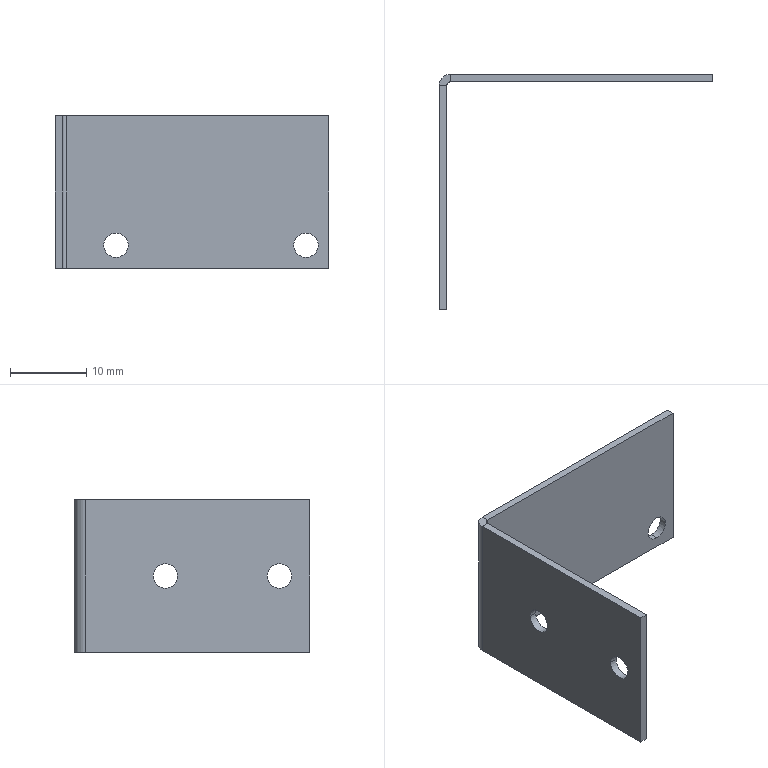Part | SolidWorks | features ICE 2, FlatPattern 1, SMBaseFlange 1, SheetMetal 1 | 1 solid | 22 faces | box 36 x 31 x 20 mm | volume 1279 mm3 | plane 12 | cylinder 10 | commonest cylinder face diameters 3.2 x8 1 x1 3 x1
STEP:
#1=CARTESIAN_POINT('',(-1.,-12.6,10.));
#2=VERTEX_POINT('',#1);
#3=CARTESIAN_POINT('',(-1.,-9.4,10.));
#4=VERTEX_POINT('',#3);
#5=CARTESIAN_POINT('',(-1.,-11.,10.));
#6=DIRECTION('',(1.,0.,0.));
#7=DIRECTION('',(0.,1.,0.));
#8=AXIS2_PLACEMENT_3D('',#5,#6,#7);
#9=CIRCLE('',#8,1.6);
#10=EDGE_CURVE('',#2,#4,#9,.T.);
#11=ORIENTED_EDGE('',*,*,#10,.F.);
#12=CARTESIAN_POINT('',(0.,-12.6,10.));
#13=VERTEX_POINT('',#12);
#14=CARTESIAN_POINT('',(-1.,-12.6,10.));
#15=DIRECTION('',(1.,0.,0.));
#16=VECTOR('',#15,1000.);
#17=LINE('',#14,#16);
#18=EDGE_CURVE('',#2,#13,#17,.T.);
#19=ORIENTED_EDGE('',*,*,#18,.T.);
#20=CARTESIAN_POINT('',(0.,-9.4,10.));
#21=VERTEX_POINT('',#20);
#22=CARTESIAN_POINT('',(0.,-11.,10.));
#23=DIRECTION('',(1.,0.,0.));
#24=DIRECTION('',(0.,1.,0.));
#25=AXIS2_PLACEMENT_3D('',#22,#23,#24);
#26=CIRCLE('',#25,1.6);
#27=EDGE_CURVE('',#13,#21,#26,.T.);
#28=ORIENTED_EDGE('',*,*,#27,.T.);
#29=CARTESIAN_POINT('',(-1.,-9.4,10.));
#30=DIRECTION('',(1.,0.,0.));
#31=VECTOR('',#30,1000.);
#32=LINE('',#29,#31);
#33=EDGE_CURVE('',#4,#21,#32,.T.);
#34=ORIENTED_EDGE('',*,*,#33,.F.);
#35=EDGE_LOOP('',(#11,#19,#28,#34));
#36=FACE_OUTER_BOUND('',#35,.T.);
#37=CARTESIAN_POINT('',(-1.,-11.,10.));
#38=DIRECTION('',(1.,0.,0.));
#39=DIRECTION('',(0.,1.,0.));
#40=AXIS2_PLACEMENT_3D('',#37,#38,#39);
#41=CYLINDRICAL_SURFACE('',#40,1.6);
#42=ADVANCED_FACE('',(#36),#41,.F.);
#43=CARTESIAN_POINT('',(-1.,-27.6,10.));
#44=VERTEX_POINT('',#43);
#45=CARTESIAN_POINT('',(-1.,-24.4,10.));
#46=VERTEX_POINT('',#45);
#47=CARTESIAN_POINT('',(-1.,-26.,10.));
#48=DIRECTION('',(1.,0.,0.));
#49=DIRECTION('',(0.,1.,0.));
#50=AXIS2_PLACEMENT_3D('',#47,#48,#49);
#51=CIRCLE('',#50,1.6);
#52=EDGE_CURVE('',#44,#46,#51,.T.);
#53=ORIENTED_EDGE('',*,*,#52,.F.);
#54=CARTESIAN_POINT('',(0.,-27.6,10.));
#55=VERTEX_POINT('',#54);
#56=CARTESIAN_POINT('',(-1.,-27.6,10.));
#57=DIRECTION('',(1.,0.,0.));
#58=VECTOR('',#57,1000.);
#59=LINE('',#56,#58);
#60=EDGE_CURVE('',#44,#55,#59,.T.);
#61=ORIENTED_EDGE('',*,*,#60,.T.);
#62=CARTESIAN_POINT('',(0.,-24.4,10.));
#63=VERTEX_POINT('',#62);
#64=CARTESIAN_POINT('',(0.,-26.,10.));
#65=DIRECTION('',(1.,0.,0.));
#66=DIRECTION('',(0.,1.,0.));
#67=AXIS2_PLACEMENT_3D('',#64,#65,#66);
#68=CIRCLE('',#67,1.6);
#69=EDGE_CURVE('',#55,#63,#68,.T.);
#70=ORIENTED_EDGE('',*,*,#69,.T.);
#71=CARTESIAN_POINT('',(-1.,-24.4,10.));
#72=DIRECTION('',(1.,0.,0.));
#73=VECTOR('',#72,1000.);
#74=LINE('',#71,#73);
#75=EDGE_CURVE('',#46,#63,#74,.T.);
#76=ORIENTED_EDGE('',*,*,#75,.F.);
#77=EDGE_LOOP('',(#53,#61,#70,#76));
#78=FACE_OUTER_BOUND('',#77,.T.);
#79=CARTESIAN_POINT('',(-1.,-26.,10.));
#80=DIRECTION('',(1.,0.,0.));
#81=DIRECTION('',(0.,1.,0.));
#82=AXIS2_PLACEMENT_3D('',#79,#80,#81);
#83=CYLINDRICAL_SURFACE('',#82,1.6);
#84=ADVANCED_FACE('',(#78),#83,.F.);
#85=CARTESIAN_POINT('',(7.,0.,4.6));
#86=VERTEX_POINT('',#85);
#87=CARTESIAN_POINT('',(7.,0.,1.4));
#88=VERTEX_POINT('',#87);
#89=CARTESIAN_POINT('',(7.,0.,3.));
#90=DIRECTION('',(0.,-1.,0.));
#91=DIRECTION('',(0.,0.,-1.));
#92=AXIS2_PLACEMENT_3D('',#89,#90,#91);
#93=CIRCLE('',#92,1.6);
#94=EDGE_CURVE('',#86,#88,#93,.T.);
#95=ORIENTED_EDGE('',*,*,#94,.T.);
#96=CARTESIAN_POINT('',(7.,1.,1.4));
#97=VERTEX_POINT('',#96);
#98=CARTESIAN_POINT('',(7.,-9.,1.4));
#99=DIRECTION('',(0.,1.,0.));
#100=VECTOR('',#99,1000.);
#101=LINE('',#98,#100);
#102=EDGE_CURVE('',#88,#97,#101,.T.);
#103=ORIENTED_EDGE('',*,*,#102,.T.);
#104=CARTESIAN_POINT('',(7.,1.,4.6));
#105=VERTEX_POINT('',#104);
#106=CARTESIAN_POINT('',(7.,1.,3.));
#107=DIRECTION('',(0.,1.,0.));
#108=DIRECTION('',(0.,0.,1.));
#109=AXIS2_PLACEMENT_3D('',#106,#107,#108);
#110=CIRCLE('',#109,1.6);
#111=EDGE_CURVE('',#97,#105,#110,.T.);
#112=ORIENTED_EDGE('',*,*,#111,.T.);
#113=CARTESIAN_POINT('',(7.,-9.,4.6));
#114=DIRECTION('',(0.,1.,0.));
#115=VECTOR('',#114,1000.);
#116=LINE('',#113,#115);
#117=EDGE_CURVE('',#86,#105,#116,.T.);
#118=ORIENTED_EDGE('',*,*,#117,.F.);
#119=EDGE_LOOP('',(#95,#103,#112,#118));
#120=FACE_OUTER_BOUND('',#119,.T.);
#121=CARTESIAN_POINT('',(7.,-9.,3.));
#122=DIRECTION('',(0.,1.,0.));
#123=DIRECTION('',(0.,0.,1.));
#124=AXIS2_PLACEMENT_3D('',#121,#122,#123);
#125=CYLINDRICAL_SURFACE('',#124,1.6);
#126=ADVANCED_FACE('',(#120),#125,.F.);
#127=CARTESIAN_POINT('',(32.,0.,4.6));
#128=VERTEX_POINT('',#127);
#129=CARTESIAN_POINT('',(32.,0.,1.4));
#130=VERTEX_POINT('',#129);
#131=CARTESIAN_POINT('',(32.,0.,3.));
#132=DIRECTION('',(0.,-1.,0.));
#133=DIRECTION('',(0.,0.,-1.));
#134=AXIS2_PLACEMENT_3D('',#131,#132,#133);
#135=CIRCLE('',#134,1.6);
#136=EDGE_CURVE('',#128,#130,#135,.T.);
#137=ORIENTED_EDGE('',*,*,#136,.T.);
#138=CARTESIAN_POINT('',(32.,1.,1.4));
#139=VERTEX_POINT('',#138);
#140=CARTESIAN_POINT('',(32.,-9.,1.4));
#141=DIRECTION('',(0.,1.,0.));
#142=VECTOR('',#141,1000.);
#143=LINE('',#140,#142);
#144=EDGE_CURVE('',#130,#139,#143,.T.);
#145=ORIENTED_EDGE('',*,*,#144,.T.);
#146=CARTESIAN_POINT('',(32.,1.,4.6));
#147=VERTEX_POINT('',#146);
#148=CARTESIAN_POINT('',(32.,1.,3.));
#149=DIRECTION('',(0.,1.,0.));
#150=DIRECTION('',(0.,0.,1.));
#151=AXIS2_PLACEMENT_3D('',#148,#149,#150);
#152=CIRCLE('',#151,1.6);
#153=EDGE_CURVE('',#139,#147,#152,.T.);
#154=ORIENTED_EDGE('',*,*,#153,.T.);
#155=CARTESIAN_POINT('',(32.,-9.,4.6));
#156=DIRECTION('',(0.,1.,0.));
#157=VECTOR('',#156,1000.);
#158=LINE('',#155,#157);
#159=EDGE_CURVE('',#128,#147,#158,.T.);
#160=ORIENTED_EDGE('',*,*,#159,.F.);
#161=EDGE_LOOP('',(#137,#145,#154,#160));
#162=FACE_OUTER_BOUND('',#161,.T.);
#163=CARTESIAN_POINT('',(32.,-9.,3.));
#164=DIRECTION('',(0.,1.,0.));
#165=DIRECTION('',(0.,0.,1.));
#166=AXIS2_PLACEMENT_3D('',#163,#164,#165);
#167=CYLINDRICAL_SURFACE('',#166,1.6);
#168=ADVANCED_FACE('',(#162),#167,.F.);
#169=CARTESIAN_POINT('',(0.,-0.5,20.));
#170=VERTEX_POINT('',#169);
#171=CARTESIAN_POINT('',(-1.,-0.5,20.));
#172=VERTEX_POINT('',#171);
#173=CARTESIAN_POINT('',(0.,-0.5,20.));
#174=DIRECTION('',(-1.,0.,0.));
#175=VECTOR('',#174,1000.);
#176=LINE('',#173,#175);
#177=EDGE_CURVE('',#170,#172,#176,.T.);
#178=ORIENTED_EDGE('',*,*,#177,.F.);
#179=CARTESIAN_POINT('',(0.5,0.,20.));
#180=VERTEX_POINT('',#179);
#181=CARTESIAN_POINT('',(0.5,-0.5,20.));
#182=DIRECTION('',(0.,0.,1.));
#183=DIRECTION('',(-1.,0.,0.));
#184=AXIS2_PLACEMENT_3D('',#181,#182,#183);
#185=CIRCLE('',#184,0.5);
#186=EDGE_CURVE('',#180,#170,#185,.T.);
#187=ORIENTED_EDGE('',*,*,#186,.F.);
#188=CARTESIAN_POINT('',(0.5,1.,20.));
#189=VERTEX_POINT('',#188);
#190=CARTESIAN_POINT('',(0.5,1.,20.));
#191=DIRECTION('',(0.,-1.,0.));
#192=VECTOR('',#191,1000.);
#193=LINE('',#190,#192);
#194=EDGE_CURVE('',#189,#180,#193,.T.);
#195=ORIENTED_EDGE('',*,*,#194,.F.);
#196=CARTESIAN_POINT('',(0.5,-0.5,20.));
#197=DIRECTION('',(0.,0.,1.));
#198=DIRECTION('',(1.,0.,0.));
#199=AXIS2_PLACEMENT_3D('',#196,#197,#198);
#200=CIRCLE('',#199,1.5);
#201=EDGE_CURVE('',#189,#172,#200,.T.);
#202=ORIENTED_EDGE('',*,*,#201,.T.);
#203=EDGE_LOOP('',(#178,#187,#195,#202));
#204=FACE_OUTER_BOUND('',#203,.T.);
#205=CARTESIAN_POINT('',(0.,-0.5,20.));
#206=DIRECTION('',(0.,0.,1.));
#207=DIRECTION('',(1.,0.,0.));
#208=AXIS2_PLACEMENT_3D('',#205,#206,#207);
#209=PLANE('',#208);
#210=ADVANCED_FACE('',(#204),#209,.T.);
#211=CARTESIAN_POINT('',(0.,-30.,20.));
#212=VERTEX_POINT('',#211);
#213=CARTESIAN_POINT('',(0.,0.,20.));
#214=DIRECTION('',(0.,-1.,0.));
#215=VECTOR('',#214,1000.);
#216=LINE('',#213,#215);
#217=EDGE_CURVE('',#170,#212,#216,.T.);
#218=ORIENTED_EDGE('',*,*,#217,.F.);
#219=ORIENTED_EDGE('',*,*,#177,.T.);
#220=CARTESIAN_POINT('',(-1.,-30.,20.));
#221=VERTEX_POINT('',#220);
#222=CARTESIAN_POINT('',(-1.,0.,20.));
#223=DIRECTION('',(0.,-1.,0.));
#224=VECTOR('',#223,1000.);
#225=LINE('',#222,#224);
#226=EDGE_CURVE('',#172,#221,#225,.T.);
#227=ORIENTED_EDGE('',*,*,#226,.T.);
#228=CARTESIAN_POINT('',(0.,-30.,20.));
#229=DIRECTION('',(-1.,0.,0.));
#230=VECTOR('',#229,1000.);
#231=LINE('',#228,#230);
#232=EDGE_CURVE('',#212,#221,#231,.T.);
#233=ORIENTED_EDGE('',*,*,#232,.F.);
#234=EDGE_LOOP('',(#218,#219,#227,#233));
#235=FACE_OUTER_BOUND('',#234,.T.);
#236=CARTESIAN_POINT('',(0.5,1.,20.));
#237=DIRECTION('',(0.,0.,1.));
#238=DIRECTION('',(1.,0.,0.));
#239=AXIS2_PLACEMENT_3D('',#236,#237,#238);
#240=PLANE('',#239);
#241=ADVANCED_FACE('',(#235),#240,.T.);
#242=CARTESIAN_POINT('',(0.5,0.,0.));
#243=VERTEX_POINT('',#242);
#244=CARTESIAN_POINT('',(0.5,1.,0.));
#245=VERTEX_POINT('',#244);
#246=CARTESIAN_POINT('',(0.5,0.,0.));
#247=DIRECTION('',(0.,1.,0.));
#248=VECTOR('',#247,1000.);
#249=LINE('',#246,#248);
#250=EDGE_CURVE('',#243,#245,#249,.T.);
#251=ORIENTED_EDGE('',*,*,#250,.F.);
#252=CARTESIAN_POINT('',(0.,-0.5,0.));
#253=VERTEX_POINT('',#252);
#254=CARTESIAN_POINT('',(0.5,-0.5,0.));
#255=DIRECTION('',(0.,0.,1.));
#256=DIRECTION('',(-1.,0.,0.));
#257=AXIS2_PLACEMENT_3D('',#254,#255,#256);
#258=CIRCLE('',#257,0.5);
#259=EDGE_CURVE('',#243,#253,#258,.T.);
#260=ORIENTED_EDGE('',*,*,#259,.T.);
#261=CARTESIAN_POINT('',(-1.,-0.5,0.));
#262=VERTEX_POINT('',#261);
#263=CARTESIAN_POINT('',(-1.,-0.5,0.));
#264=DIRECTION('',(1.,0.,0.));
#265=VECTOR('',#264,1000.);
#266=LINE('',#263,#265);
#267=EDGE_CURVE('',#262,#253,#266,.T.);
#268=ORIENTED_EDGE('',*,*,#267,.F.);
#269=CARTESIAN_POINT('',(0.5,-0.5,0.));
#270=DIRECTION('',(0.,0.,1.));
#271=DIRECTION('',(1.,0.,0.));
#272=AXIS2_PLACEMENT_3D('',#269,#270,#271);
#273=CIRCLE('',#272,1.5);
#274=EDGE_CURVE('',#245,#262,#273,.T.);
#275=ORIENTED_EDGE('',*,*,#274,.F.);
#276=EDGE_LOOP('',(#251,#260,#268,#275));
#277=FACE_OUTER_BOUND('',#276,.T.);
#278=CARTESIAN_POINT('',(0.5,0.,0.));
#279=DIRECTION('',(0.,0.,-1.));
#280=DIRECTION('',(-1.,0.,0.));
#281=AXIS2_PLACEMENT_3D('',#278,#279,#280);
#282=PLANE('',#281);
#283=ADVANCED_FACE('',(#277),#282,.T.);
#284=CARTESIAN_POINT('',(35.,0.,0.));
#285=VERTEX_POINT('',#284);
#286=CARTESIAN_POINT('',(0.,0.,0.));
#287=DIRECTION('',(-1.,0.,0.));
#288=VECTOR('',#287,1000.);
#289=LINE('',#286,#288);
#290=EDGE_CURVE('',#285,#243,#289,.T.);
#291=ORIENTED_EDGE('',*,*,#290,.T.);
#292=ORIENTED_EDGE('',*,*,#250,.T.);
#293=CARTESIAN_POINT('',(35.,1.,0.));
#294=VERTEX_POINT('',#293);
#295=CARTESIAN_POINT('',(0.,1.,0.));
#296=DIRECTION('',(-1.,0.,0.));
#297=VECTOR('',#296,1000.);
#298=LINE('',#295,#297);
#299=EDGE_CURVE('',#294,#245,#298,.T.);
#300=ORIENTED_EDGE('',*,*,#299,.F.);
#301=CARTESIAN_POINT('',(35.,1.,0.));
#302=DIRECTION('',(0.,-1.,0.));
#303=VECTOR('',#302,1000.);
#304=LINE('',#301,#303);
#305=EDGE_CURVE('',#294,#285,#304,.T.);
#306=ORIENTED_EDGE('',*,*,#305,.T.);
#307=EDGE_LOOP('',(#291,#292,#300,#306));
#308=FACE_OUTER_BOUND('',#307,.T.);
#309=CARTESIAN_POINT('',(-1.,-0.5,0.));
#310=DIRECTION('',(0.,0.,-1.));
#311=DIRECTION('',(-1.,0.,0.));
#312=AXIS2_PLACEMENT_3D('',#309,#310,#311);
#313=PLANE('',#312);
#314=ADVANCED_FACE('',(#308),#313,.T.);
#315=CARTESIAN_POINT('',(-1.,-11.,10.));
#316=DIRECTION('',(1.,0.,0.));
#317=DIRECTION('',(0.,1.,0.));
#318=AXIS2_PLACEMENT_3D('',#315,#316,#317);
#319=CIRCLE('',#318,1.6);
#320=EDGE_CURVE('',#4,#2,#319,.T.);
#321=ORIENTED_EDGE('',*,*,#320,.T.);
#322=ORIENTED_EDGE('',*,*,#10,.T.);
#323=EDGE_LOOP('',(#321,#322));
#324=FACE_BOUND('',#323,.T.);
#325=CARTESIAN_POINT('',(-1.,-26.,10.));
#326=DIRECTION('',(1.,0.,0.));
#327=DIRECTION('',(0.,1.,0.));
#328=AXIS2_PLACEMENT_3D('',#325,#326,#327);
#329=CIRCLE('',#328,1.6);
#330=EDGE_CURVE('',#46,#44,#329,.T.);
#331=ORIENTED_EDGE('',*,*,#330,.T.);
#332=ORIENTED_EDGE('',*,*,#52,.T.);
#333=EDGE_LOOP('',(#331,#332));
#334=FACE_BOUND('',#333,.T.);
#335=CARTESIAN_POINT('',(-1.,-30.,0.));
#336=VERTEX_POINT('',#335);
#337=CARTESIAN_POINT('',(-1.,0.,0.));
#338=DIRECTION('',(0.,-1.,0.));
#339=VECTOR('',#338,1000.);
#340=LINE('',#337,#339);
#341=EDGE_CURVE('',#262,#336,#340,.T.);
#342=ORIENTED_EDGE('',*,*,#341,.T.);
#343=CARTESIAN_POINT('',(-1.,-30.,20.));
#344=DIRECTION('',(0.,0.,-1.));
#345=VECTOR('',#344,1000.);
#346=LINE('',#343,#345);
#347=EDGE_CURVE('',#221,#336,#346,.T.);
#348=ORIENTED_EDGE('',*,*,#347,.F.);
#349=ORIENTED_EDGE('',*,*,#226,.F.);
#350=CARTESIAN_POINT('',(-1.,-0.5,20.));
#351=DIRECTION('',(0.,0.,-1.));
#352=VECTOR('',#351,1000.);
#353=LINE('',#350,#352);
#354=EDGE_CURVE('',#172,#262,#353,.T.);
#355=ORIENTED_EDGE('',*,*,#354,.T.);
#356=EDGE_LOOP('',(#342,#348,#349,#355));
#357=FACE_OUTER_BOUND('',#356,.T.);
#358=CARTESIAN_POINT('',(-1.,0.,20.));
#359=DIRECTION('',(1.,0.,0.));
#360=DIRECTION('',(0.,1.,0.));
#361=AXIS2_PLACEMENT_3D('',#358,#359,#360);
#362=PLANE('',#361);
#363=ADVANCED_FACE('',(#324,#334,#357),#362,.F.);
#364=CARTESIAN_POINT('',(0.,-30.,0.));
#365=VERTEX_POINT('',#364);
#366=CARTESIAN_POINT('',(0.,-30.,0.));
#367=DIRECTION('',(-1.,0.,0.));
#368=VECTOR('',#367,1000.);
#369=LINE('',#366,#368);
#370=EDGE_CURVE('',#365,#336,#369,.T.);
#371=ORIENTED_EDGE('',*,*,#370,.F.);
#372=CARTESIAN_POINT('',(0.,-30.,20.));
#373=DIRECTION('',(0.,0.,-1.));
#374=VECTOR('',#373,1000.);
#375=LINE('',#372,#374);
#376=EDGE_CURVE('',#212,#365,#375,.T.);
#377=ORIENTED_EDGE('',*,*,#376,.F.);
#378=ORIENTED_EDGE('',*,*,#232,.T.);
#379=ORIENTED_EDGE('',*,*,#347,.T.);
#380=EDGE_LOOP('',(#371,#377,#378,#379));
#381=FACE_OUTER_BOUND('',#380,.T.);
#382=CARTESIAN_POINT('',(0.,-30.,20.));
#383=DIRECTION('',(0.,-1.,0.));
#384=DIRECTION('',(0.,0.,-1.));
#385=AXIS2_PLACEMENT_3D('',#382,#383,#384);
#386=PLANE('',#385);
#387=ADVANCED_FACE('',(#381),#386,.T.);
#388=CARTESIAN_POINT('',(0.,-11.,10.));
#389=DIRECTION('',(1.,0.,0.));
#390=DIRECTION('',(0.,1.,0.));
#391=AXIS2_PLACEMENT_3D('',#388,#389,#390);
#392=CIRCLE('',#391,1.6);
#393=EDGE_CURVE('',#21,#13,#392,.T.);
#394=ORIENTED_EDGE('',*,*,#393,.F.);
#395=ORIENTED_EDGE('',*,*,#27,.F.);
#396=EDGE_LOOP('',(#394,#395));
#397=FACE_BOUND('',#396,.T.);
#398=CARTESIAN_POINT('',(0.,-26.,10.));
#399=DIRECTION('',(1.,0.,0.));
#400=DIRECTION('',(0.,1.,0.));
#401=AXIS2_PLACEMENT_3D('',#398,#399,#400);
#402=CIRCLE('',#401,1.6);
#403=EDGE_CURVE('',#63,#55,#402,.T.);
#404=ORIENTED_EDGE('',*,*,#403,.F.);
#405=ORIENTED_EDGE('',*,*,#69,.F.);
#406=EDGE_LOOP('',(#404,#405));
#407=FACE_BOUND('',#406,.T.);
#408=CARTESIAN_POINT('',(0.,0.,0.));
#409=DIRECTION('',(0.,-1.,0.));
#410=VECTOR('',#409,1000.);
#411=LINE('',#408,#410);
#412=EDGE_CURVE('',#253,#365,#411,.T.);
#413=ORIENTED_EDGE('',*,*,#412,.F.);
#414=CARTESIAN_POINT('',(0.,-0.5,20.));
#415=DIRECTION('',(0.,0.,-1.));
#416=VECTOR('',#415,1000.);
#417=LINE('',#414,#416);
#418=EDGE_CURVE('',#170,#253,#417,.T.);
#419=ORIENTED_EDGE('',*,*,#418,.F.);
#420=ORIENTED_EDGE('',*,*,#217,.T.);
#421=ORIENTED_EDGE('',*,*,#376,.T.);
#422=EDGE_LOOP('',(#413,#419,#420,#421));
#423=FACE_OUTER_BOUND('',#422,.T.);
#424=CARTESIAN_POINT('',(0.,0.,20.));
#425=DIRECTION('',(1.,0.,0.));
#426=DIRECTION('',(0.,1.,0.));
#427=AXIS2_PLACEMENT_3D('',#424,#425,#426);
#428=PLANE('',#427);
#429=ADVANCED_FACE('',(#397,#407,#423),#428,.T.);
#430=ORIENTED_EDGE('',*,*,#259,.F.);
#431=CARTESIAN_POINT('',(0.5,0.,20.));
#432=DIRECTION('',(0.,0.,-1.));
#433=VECTOR('',#432,1000.);
#434=LINE('',#431,#433);
#435=EDGE_CURVE('',#180,#243,#434,.T.);
#436=ORIENTED_EDGE('',*,*,#435,.F.);
#437=ORIENTED_EDGE('',*,*,#186,.T.);
#438=ORIENTED_EDGE('',*,*,#418,.T.);
#439=EDGE_LOOP('',(#430,#436,#437,#438));
#440=FACE_OUTER_BOUND('',#439,.T.);
#441=CARTESIAN_POINT('',(0.5,-0.5,20.));
#442=DIRECTION('',(0.,0.,-1.));
#443=DIRECTION('',(-1.,0.,0.));
#444=AXIS2_PLACEMENT_3D('',#441,#442,#443);
#445=CYLINDRICAL_SURFACE('',#444,0.5);
#446=ADVANCED_FACE('',(#440),#445,.F.);
#447=ORIENTED_EDGE('',*,*,#94,.F.);
#448=CARTESIAN_POINT('',(7.,0.,3.));
#449=DIRECTION('',(0.,-1.,0.));
#450=DIRECTION('',(0.,0.,-1.));
#451=AXIS2_PLACEMENT_3D('',#448,#449,#450);
#452=CIRCLE('',#451,1.6);
#453=EDGE_CURVE('',#88,#86,#452,.T.);
#454=ORIENTED_EDGE('',*,*,#453,.F.);
#455=EDGE_LOOP('',(#447,#454));
#456=FACE_BOUND('',#455,.T.);
#457=ORIENTED_EDGE('',*,*,#136,.F.);
#458=CARTESIAN_POINT('',(32.,0.,3.));
#459=DIRECTION('',(0.,-1.,0.));
#460=DIRECTION('',(0.,0.,-1.));
#461=AXIS2_PLACEMENT_3D('',#458,#459,#460);
#462=CIRCLE('',#461,1.6);
#463=EDGE_CURVE('',#130,#128,#462,.T.);
#464=ORIENTED_EDGE('',*,*,#463,.F.);
#465=EDGE_LOOP('',(#457,#464));
#466=FACE_BOUND('',#465,.T.);
#467=ORIENTED_EDGE('',*,*,#290,.F.);
#468=CARTESIAN_POINT('',(35.,0.,20.));
#469=VERTEX_POINT('',#468);
#470=CARTESIAN_POINT('',(35.,0.,20.));
#471=DIRECTION('',(0.,0.,-1.));
#472=VECTOR('',#471,1000.);
#473=LINE('',#470,#472);
#474=EDGE_CURVE('',#469,#285,#473,.T.);
#475=ORIENTED_EDGE('',*,*,#474,.F.);
#476=CARTESIAN_POINT('',(0.,0.,20.));
#477=DIRECTION('',(-1.,0.,0.));
#478=VECTOR('',#477,1000.);
#479=LINE('',#476,#478);
#480=EDGE_CURVE('',#469,#180,#479,.T.);
#481=ORIENTED_EDGE('',*,*,#480,.T.);
#482=ORIENTED_EDGE('',*,*,#435,.T.);
#483=EDGE_LOOP('',(#467,#475,#481,#482));
#484=FACE_OUTER_BOUND('',#483,.T.);
#485=CARTESIAN_POINT('',(0.,0.,20.));
#486=DIRECTION('',(0.,-1.,0.));
#487=DIRECTION('',(0.,0.,-1.));
#488=AXIS2_PLACEMENT_3D('',#485,#486,#487);
#489=PLANE('',#488);
#490=ADVANCED_FACE('',(#456,#466,#484),#489,.T.);
#491=ORIENTED_EDGE('',*,*,#305,.F.);
#492=CARTESIAN_POINT('',(35.,1.,20.));
#493=VERTEX_POINT('',#492);
#494=CARTESIAN_POINT('',(35.,1.,20.));
#495=DIRECTION('',(0.,0.,-1.));
#496=VECTOR('',#495,1000.);
#497=LINE('',#494,#496);
#498=EDGE_CURVE('',#493,#294,#497,.T.);
#499=ORIENTED_EDGE('',*,*,#498,.F.);
#500=CARTESIAN_POINT('',(35.,1.,20.));
#501=DIRECTION('',(0.,-1.,0.));
#502=VECTOR('',#501,1000.);
#503=LINE('',#500,#502);
#504=EDGE_CURVE('',#493,#469,#503,.T.);
#505=ORIENTED_EDGE('',*,*,#504,.T.);
#506=ORIENTED_EDGE('',*,*,#474,.T.);
#507=EDGE_LOOP('',(#491,#499,#505,#506));
#508=FACE_OUTER_BOUND('',#507,.T.);
#509=CARTESIAN_POINT('',(35.,1.,20.));
#510=DIRECTION('',(1.,0.,0.));
#511=DIRECTION('',(0.,0.,-1.));
#512=AXIS2_PLACEMENT_3D('',#509,#510,#511);
#513=PLANE('',#512);
#514=ADVANCED_FACE('',(#508),#513,.T.);
#515=CARTESIAN_POINT('',(7.,1.,3.));
#516=DIRECTION('',(0.,1.,0.));
#517=DIRECTION('',(0.,0.,1.));
#518=AXIS2_PLACEMENT_3D('',#515,#516,#517);
#519=CIRCLE('',#518,1.6);
#520=EDGE_CURVE('',#105,#97,#519,.T.);
#521=ORIENTED_EDGE('',*,*,#520,.F.);
#522=ORIENTED_EDGE('',*,*,#111,.F.);
#523=EDGE_LOOP('',(#521,#522));
#524=FACE_BOUND('',#523,.T.);
#525=CARTESIAN_POINT('',(32.,1.,3.));
#526=DIRECTION('',(0.,1.,0.));
#527=DIRECTION('',(0.,0.,1.));
#528=AXIS2_PLACEMENT_3D('',#525,#526,#527);
#529=CIRCLE('',#528,1.6);
#530=EDGE_CURVE('',#147,#139,#529,.T.);
#531=ORIENTED_EDGE('',*,*,#530,.F.);
#532=ORIENTED_EDGE('',*,*,#153,.F.);
#533=EDGE_LOOP('',(#531,#532));
#534=FACE_BOUND('',#533,.T.);
#535=ORIENTED_EDGE('',*,*,#299,.T.);
#536=CARTESIAN_POINT('',(0.5,1.,20.));
#537=DIRECTION('',(0.,0.,-1.));
#538=VECTOR('',#537,1000.);
#539=LINE('',#536,#538);
#540=EDGE_CURVE('',#189,#245,#539,.T.);
#541=ORIENTED_EDGE('',*,*,#540,.F.);
#542=CARTESIAN_POINT('',(0.,1.,20.));
#543=DIRECTION('',(-1.,0.,0.));
#544=VECTOR('',#543,1000.);
#545=LINE('',#542,#544);
#546=EDGE_CURVE('',#493,#189,#545,.T.);
#547=ORIENTED_EDGE('',*,*,#546,.F.);
#548=ORIENTED_EDGE('',*,*,#498,.T.);
#549=EDGE_LOOP('',(#535,#541,#547,#548));
#550=FACE_OUTER_BOUND('',#549,.T.);
#551=CARTESIAN_POINT('',(0.,1.,20.));
#552=DIRECTION('',(0.,-1.,0.));
#553=DIRECTION('',(0.,0.,-1.));
#554=AXIS2_PLACEMENT_3D('',#551,#552,#553);
#555=PLANE('',#554);
#556=ADVANCED_FACE('',(#524,#534,#550),#555,.F.);
#557=ORIENTED_EDGE('',*,*,#274,.T.);
#558=ORIENTED_EDGE('',*,*,#354,.F.);
#559=ORIENTED_EDGE('',*,*,#201,.F.);
#560=ORIENTED_EDGE('',*,*,#540,.T.);
#561=EDGE_LOOP('',(#557,#558,#559,#560));
#562=FACE_OUTER_BOUND('',#561,.T.);
#563=CARTESIAN_POINT('',(0.5,-0.5,20.));
#564=DIRECTION('',(0.,0.,-1.));
#565=DIRECTION('',(-1.,0.,0.));
#566=AXIS2_PLACEMENT_3D('',#563,#564,#565);
#567=CYLINDRICAL_SURFACE('',#566,1.5);
#568=ADVANCED_FACE('',(#562),#567,.T.);
#569=ORIENTED_EDGE('',*,*,#546,.T.);
#570=ORIENTED_EDGE('',*,*,#194,.T.);
#571=ORIENTED_EDGE('',*,*,#480,.F.);
#572=ORIENTED_EDGE('',*,*,#504,.F.);
#573=EDGE_LOOP('',(#569,#570,#571,#572));
#574=FACE_OUTER_BOUND('',#573,.T.);
#575=CARTESIAN_POINT('',(0.5,-0.5,20.));
#576=DIRECTION('',(0.,0.,-1.));
#577=DIRECTION('',(-1.,0.,0.));
#578=AXIS2_PLACEMENT_3D('',#575,#576,#577);
#579=PLANE('',#578);
#580=ADVANCED_FACE('',(#574),#579,.F.);
#581=ORIENTED_EDGE('',*,*,#341,.F.);
#582=ORIENTED_EDGE('',*,*,#267,.T.);
#583=ORIENTED_EDGE('',*,*,#412,.T.);
#584=ORIENTED_EDGE('',*,*,#370,.T.);
#585=EDGE_LOOP('',(#581,#582,#583,#584));
#586=FACE_OUTER_BOUND('',#585,.T.);
#587=CARTESIAN_POINT('',(0.5,-0.5,0.));
#588=DIRECTION('',(0.,0.,-1.));
#589=DIRECTION('',(-1.,0.,0.));
#590=AXIS2_PLACEMENT_3D('',#587,#588,#589);
#591=PLANE('',#590);
#592=ADVANCED_FACE('',(#586),#591,.T.);
#593=ORIENTED_EDGE('',*,*,#144,.F.);
#594=ORIENTED_EDGE('',*,*,#463,.T.);
#595=ORIENTED_EDGE('',*,*,#159,.T.);
#596=ORIENTED_EDGE('',*,*,#530,.T.);
#597=EDGE_LOOP('',(#593,#594,#595,#596));
#598=FACE_OUTER_BOUND('',#597,.T.);
#599=CARTESIAN_POINT('',(32.,-9.,3.));
#600=DIRECTION('',(0.,1.,0.));
#601=DIRECTION('',(0.,0.,1.));
#602=AXIS2_PLACEMENT_3D('',#599,#600,#601);
#603=CYLINDRICAL_SURFACE('',#602,1.6);
#604=ADVANCED_FACE('',(#598),#603,.F.);
#605=ORIENTED_EDGE('',*,*,#102,.F.);
#606=ORIENTED_EDGE('',*,*,#453,.T.);
#607=ORIENTED_EDGE('',*,*,#117,.T.);
#608=ORIENTED_EDGE('',*,*,#520,.T.);
#609=EDGE_LOOP('',(#605,#606,#607,#608));
#610=FACE_OUTER_BOUND('',#609,.T.);
#611=CARTESIAN_POINT('',(7.,-9.,3.));
#612=DIRECTION('',(0.,1.,0.));
#613=DIRECTION('',(0.,0.,1.));
#614=AXIS2_PLACEMENT_3D('',#611,#612,#613);
#615=CYLINDRICAL_SURFACE('',#614,1.6);
#616=ADVANCED_FACE('',(#610),#615,.F.);
#617=ORIENTED_EDGE('',*,*,#60,.F.);
#618=ORIENTED_EDGE('',*,*,#330,.F.);
#619=ORIENTED_EDGE('',*,*,#75,.T.);
#620=ORIENTED_EDGE('',*,*,#403,.T.);
#621=EDGE_LOOP('',(#617,#618,#619,#620));
#622=FACE_OUTER_BOUND('',#621,.T.);
#623=CARTESIAN_POINT('',(-1.,-26.,10.));
#624=DIRECTION('',(1.,0.,0.));
#625=DIRECTION('',(0.,1.,0.));
#626=AXIS2_PLACEMENT_3D('',#623,#624,#625);
#627=CYLINDRICAL_SURFACE('',#626,1.6);
#628=ADVANCED_FACE('',(#622),#627,.F.);
#629=ORIENTED_EDGE('',*,*,#18,.F.);
#630=ORIENTED_EDGE('',*,*,#320,.F.);
#631=ORIENTED_EDGE('',*,*,#33,.T.);
#632=ORIENTED_EDGE('',*,*,#393,.T.);
#633=EDGE_LOOP('',(#629,#630,#631,#632));
#634=FACE_OUTER_BOUND('',#633,.T.);
#635=CARTESIAN_POINT('',(-1.,-11.,10.));
#636=DIRECTION('',(1.,0.,0.));
#637=DIRECTION('',(0.,1.,0.));
#638=AXIS2_PLACEMENT_3D('',#635,#636,#637);
#639=CYLINDRICAL_SURFACE('',#638,1.6);
#640=ADVANCED_FACE('',(#634),#639,.F.);
#641=CLOSED_SHELL('',(#42,#84,#126,#168,#210,#241,#283,#314,#363,#387,#429,#446,#490,#514,#556,#568,#580,#592,#604,#616,#628,#640));
#642=MANIFOLD_SOLID_BREP('',#641);
#643=CARTESIAN_POINT('',(0.,0.,0.));
#644=DIRECTION('',(0.,0.,1.));
#645=DIRECTION('',(1.,0.,0.));
#646=AXIS2_PLACEMENT_3D('',#643,#644,#645);
#647=(LENGTH_UNIT()NAMED_UNIT(*)SI_UNIT(.MILLI.,.METRE.));
#648=UNCERTAINTY_MEASURE_WITH_UNIT(LENGTH_MEASURE(0.00001),#647,'','');
#649=(NAMED_UNIT(*)PLANE_ANGLE_UNIT()SI_UNIT($,.RADIAN.));
#650=(NAMED_UNIT(*)SI_UNIT($,.STERADIAN.)SOLID_ANGLE_UNIT());
#651=(GEOMETRIC_REPRESENTATION_CONTEXT(3)GLOBAL_UNCERTAINTY_ASSIGNED_CONTEXT((#648))GLOBAL_UNIT_ASSIGNED_CONTEXT((#647,#649,#650))REPRESENTATION_CONTEXT('',''));
#652=ADVANCED_BREP_SHAPE_REPRESENTATION('',(#642,#646),#651);